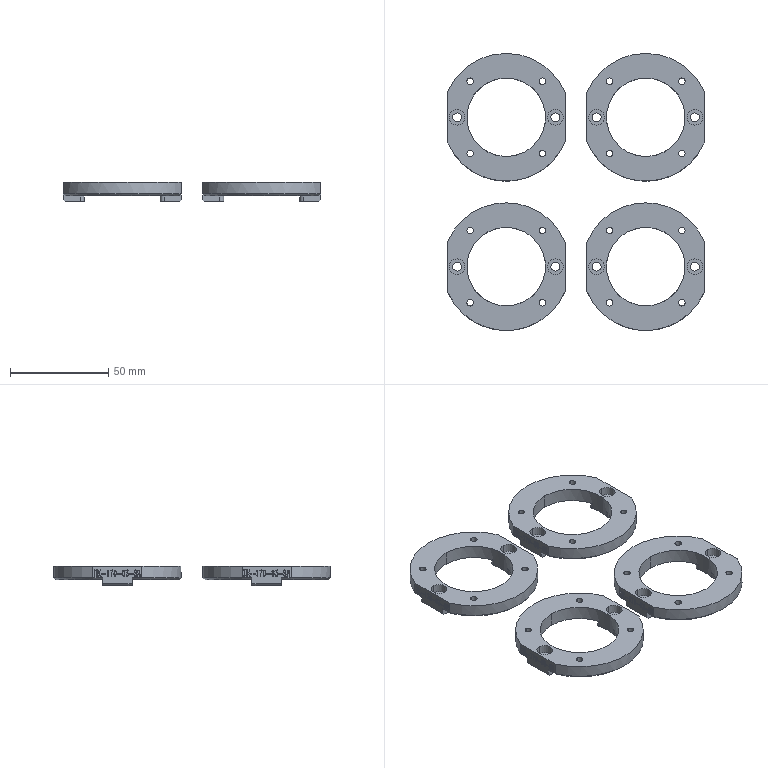Part | 4 solids | 1032 faces | box 131 x 141 x 10 mm | volume 55222 mm3 | plane 576 | spline 344 | cylinder 100 | cone 12 | commonest cylinder face diameters 3.3 x32 4 x16 4.5 x16 8 x16 65 x12 40 x8